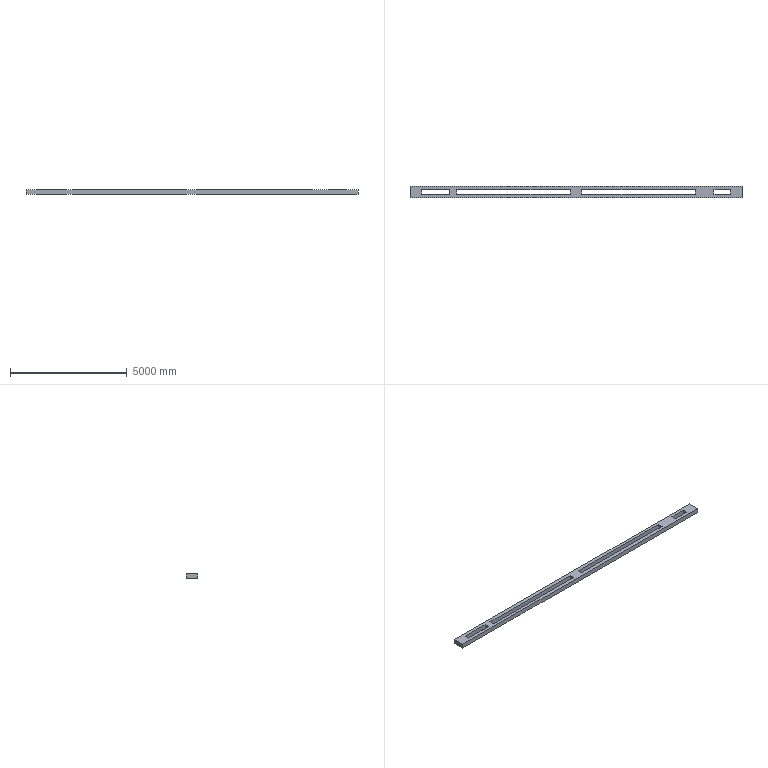Part | SolidWorks | features ICE 2, Extrusion 1 | 1 solid | 22 faces | box 14220 x 500 x 200 mm | volume 957200000 mm3 | plane 22
STEP:
#1=CARTESIAN_POINT('',(-7110.,250.,0.));
#2=VERTEX_POINT('',#1);
#3=CARTESIAN_POINT('',(-7110.,-250.,0.));
#4=VERTEX_POINT('',#3);
#5=CARTESIAN_POINT('',(-7110.,-250.,0.));
#6=DIRECTION('',(0.,-1.,0.));
#7=VECTOR('',#6,1000.);
#8=LINE('',#5,#7);
#9=EDGE_CURVE('',#2,#4,#8,.T.);
#10=ORIENTED_EDGE('',*,*,#9,.T.);
#11=CARTESIAN_POINT('',(-7110.,-250.,200.));
#12=VERTEX_POINT('',#11);
#13=CARTESIAN_POINT('',(-7110.,-250.,200.));
#14=DIRECTION('',(0.,0.,-1.));
#15=VECTOR('',#14,1000.);
#16=LINE('',#13,#15);
#17=EDGE_CURVE('',#12,#4,#16,.T.);
#18=ORIENTED_EDGE('',*,*,#17,.F.);
#19=CARTESIAN_POINT('',(-7110.,250.,200.));
#20=VERTEX_POINT('',#19);
#21=CARTESIAN_POINT('',(-7110.,-250.,200.));
#22=DIRECTION('',(0.,-1.,0.));
#23=VECTOR('',#22,1000.);
#24=LINE('',#21,#23);
#25=EDGE_CURVE('',#20,#12,#24,.T.);
#26=ORIENTED_EDGE('',*,*,#25,.F.);
#27=CARTESIAN_POINT('',(-7110.,250.,200.));
#28=DIRECTION('',(0.,0.,-1.));
#29=VECTOR('',#28,1000.);
#30=LINE('',#27,#29);
#31=EDGE_CURVE('',#20,#2,#30,.T.);
#32=ORIENTED_EDGE('',*,*,#31,.T.);
#33=EDGE_LOOP('',(#10,#18,#26,#32));
#34=FACE_OUTER_BOUND('',#33,.T.);
#35=CARTESIAN_POINT('',(-7110.,-250.,200.));
#36=DIRECTION('',(1.,0.,0.));
#37=DIRECTION('',(0.,0.,-1.));
#38=AXIS2_PLACEMENT_3D('',#35,#36,#37);
#39=PLANE('',#38);
#40=ADVANCED_FACE('',(#34),#39,.F.);
#41=CARTESIAN_POINT('',(7110.,-250.,0.));
#42=VERTEX_POINT('',#41);
#43=CARTESIAN_POINT('',(7110.,-250.,0.));
#44=DIRECTION('',(1.,0.,0.));
#45=VECTOR('',#44,1000.);
#46=LINE('',#43,#45);
#47=EDGE_CURVE('',#4,#42,#46,.T.);
#48=ORIENTED_EDGE('',*,*,#47,.T.);
#49=CARTESIAN_POINT('',(7110.,-250.,200.));
#50=VERTEX_POINT('',#49);
#51=CARTESIAN_POINT('',(7110.,-250.,200.));
#52=DIRECTION('',(0.,0.,-1.));
#53=VECTOR('',#52,1000.);
#54=LINE('',#51,#53);
#55=EDGE_CURVE('',#50,#42,#54,.T.);
#56=ORIENTED_EDGE('',*,*,#55,.F.);
#57=CARTESIAN_POINT('',(7110.,-250.,200.));
#58=DIRECTION('',(1.,0.,0.));
#59=VECTOR('',#58,1000.);
#60=LINE('',#57,#59);
#61=EDGE_CURVE('',#12,#50,#60,.T.);
#62=ORIENTED_EDGE('',*,*,#61,.F.);
#63=ORIENTED_EDGE('',*,*,#17,.T.);
#64=EDGE_LOOP('',(#48,#56,#62,#63));
#65=FACE_OUTER_BOUND('',#64,.T.);
#66=CARTESIAN_POINT('',(7110.,-250.,200.));
#67=DIRECTION('',(0.,1.,0.));
#68=DIRECTION('',(-1.,0.,0.));
#69=AXIS2_PLACEMENT_3D('',#66,#67,#68);
#70=PLANE('',#69);
#71=ADVANCED_FACE('',(#65),#70,.F.);
#72=CARTESIAN_POINT('',(7110.,250.,0.));
#73=VERTEX_POINT('',#72);
#74=CARTESIAN_POINT('',(7110.,-250.,0.));
#75=DIRECTION('',(0.,1.,0.));
#76=VECTOR('',#75,1000.);
#77=LINE('',#74,#76);
#78=EDGE_CURVE('',#42,#73,#77,.T.);
#79=ORIENTED_EDGE('',*,*,#78,.T.);
#80=CARTESIAN_POINT('',(7110.,250.,200.));
#81=VERTEX_POINT('',#80);
#82=CARTESIAN_POINT('',(7110.,250.,200.));
#83=DIRECTION('',(0.,0.,-1.));
#84=VECTOR('',#83,1000.);
#85=LINE('',#82,#84);
#86=EDGE_CURVE('',#81,#73,#85,.T.);
#87=ORIENTED_EDGE('',*,*,#86,.F.);
#88=CARTESIAN_POINT('',(7110.,-250.,200.));
#89=DIRECTION('',(0.,1.,0.));
#90=VECTOR('',#89,1000.);
#91=LINE('',#88,#90);
#92=EDGE_CURVE('',#50,#81,#91,.T.);
#93=ORIENTED_EDGE('',*,*,#92,.F.);
#94=ORIENTED_EDGE('',*,*,#55,.T.);
#95=EDGE_LOOP('',(#79,#87,#93,#94));
#96=FACE_OUTER_BOUND('',#95,.T.);
#97=CARTESIAN_POINT('',(7110.,-250.,200.));
#98=DIRECTION('',(-1.,0.,0.));
#99=DIRECTION('',(0.,0.,1.));
#100=AXIS2_PLACEMENT_3D('',#97,#98,#99);
#101=PLANE('',#100);
#102=ADVANCED_FACE('',(#96),#101,.F.);
#103=CARTESIAN_POINT('',(7110.,250.,0.));
#104=DIRECTION('',(-1.,0.,0.));
#105=VECTOR('',#104,1000.);
#106=LINE('',#103,#105);
#107=EDGE_CURVE('',#73,#2,#106,.T.);
#108=ORIENTED_EDGE('',*,*,#107,.T.);
#109=ORIENTED_EDGE('',*,*,#31,.F.);
#110=CARTESIAN_POINT('',(7110.,250.,200.));
#111=DIRECTION('',(-1.,0.,0.));
#112=VECTOR('',#111,1000.);
#113=LINE('',#110,#112);
#114=EDGE_CURVE('',#81,#20,#113,.T.);
#115=ORIENTED_EDGE('',*,*,#114,.F.);
#116=ORIENTED_EDGE('',*,*,#86,.T.);
#117=EDGE_LOOP('',(#108,#109,#115,#116));
#118=FACE_OUTER_BOUND('',#117,.T.);
#119=CARTESIAN_POINT('',(7110.,250.,200.));
#120=DIRECTION('',(0.,-1.,0.));
#121=DIRECTION('',(1.,0.,0.));
#122=AXIS2_PLACEMENT_3D('',#119,#120,#121);
#123=PLANE('',#122);
#124=ADVANCED_FACE('',(#118),#123,.F.);
#125=CARTESIAN_POINT('',(5910.,-100.,200.));
#126=VERTEX_POINT('',#125);
#127=CARTESIAN_POINT('',(6610.,-100.,200.));
#128=VERTEX_POINT('',#127);
#129=CARTESIAN_POINT('',(6610.,-100.,200.));
#130=DIRECTION('',(1.,0.,0.));
#131=VECTOR('',#130,1000.);
#132=LINE('',#129,#131);
#133=EDGE_CURVE('',#126,#128,#132,.T.);
#134=ORIENTED_EDGE('',*,*,#133,.F.);
#135=CARTESIAN_POINT('',(5910.,100.,200.));
#136=VERTEX_POINT('',#135);
#137=CARTESIAN_POINT('',(5910.,100.,200.));
#138=DIRECTION('',(0.,1.,0.));
#139=VECTOR('',#138,1000.);
#140=LINE('',#137,#139);
#141=EDGE_CURVE('',#126,#136,#140,.T.);
#142=ORIENTED_EDGE('',*,*,#141,.T.);
#143=CARTESIAN_POINT('',(6610.,100.,200.));
#144=VERTEX_POINT('',#143);
#145=CARTESIAN_POINT('',(6610.,100.,200.));
#146=DIRECTION('',(-1.,0.,0.));
#147=VECTOR('',#146,1000.);
#148=LINE('',#145,#147);
#149=EDGE_CURVE('',#144,#136,#148,.T.);
#150=ORIENTED_EDGE('',*,*,#149,.F.);
#151=CARTESIAN_POINT('',(6610.,100.,200.));
#152=DIRECTION('',(0.,1.,0.));
#153=VECTOR('',#152,1000.);
#154=LINE('',#151,#153);
#155=EDGE_CURVE('',#128,#144,#154,.T.);
#156=ORIENTED_EDGE('',*,*,#155,.F.);
#157=EDGE_LOOP('',(#134,#142,#150,#156));
#158=FACE_BOUND('',#157,.T.);
#159=CARTESIAN_POINT('',(-6610.,100.,200.));
#160=VERTEX_POINT('',#159);
#161=CARTESIAN_POINT('',(-6610.,-100.,200.));
#162=VERTEX_POINT('',#161);
#163=CARTESIAN_POINT('',(-6610.,100.,200.));
#164=DIRECTION('',(0.,-1.,0.));
#165=VECTOR('',#164,1000.);
#166=LINE('',#163,#165);
#167=EDGE_CURVE('',#160,#162,#166,.T.);
#168=ORIENTED_EDGE('',*,*,#167,.F.);
#169=CARTESIAN_POINT('',(-5410.,100.,200.));
#170=VERTEX_POINT('',#169);
#171=CARTESIAN_POINT('',(-6610.,100.,200.));
#172=DIRECTION('',(-1.,0.,0.));
#173=VECTOR('',#172,1000.);
#174=LINE('',#171,#173);
#175=EDGE_CURVE('',#170,#160,#174,.T.);
#176=ORIENTED_EDGE('',*,*,#175,.F.);
#177=CARTESIAN_POINT('',(-5410.,-100.,200.));
#178=VERTEX_POINT('',#177);
#179=CARTESIAN_POINT('',(-5410.,100.,200.));
#180=DIRECTION('',(0.,1.,0.));
#181=VECTOR('',#180,1000.);
#182=LINE('',#179,#181);
#183=EDGE_CURVE('',#178,#170,#182,.T.);
#184=ORIENTED_EDGE('',*,*,#183,.F.);
#185=CARTESIAN_POINT('',(-6610.,-100.,200.));
#186=DIRECTION('',(1.,0.,0.));
#187=VECTOR('',#186,1000.);
#188=LINE('',#185,#187);
#189=EDGE_CURVE('',#162,#178,#188,.T.);
#190=ORIENTED_EDGE('',*,*,#189,.F.);
#191=EDGE_LOOP('',(#168,#176,#184,#190));
#192=FACE_BOUND('',#191,.T.);
#193=CARTESIAN_POINT('',(-5110.,100.,200.));
#194=VERTEX_POINT('',#193);
#195=CARTESIAN_POINT('',(-5110.,-100.,200.));
#196=VERTEX_POINT('',#195);
#197=CARTESIAN_POINT('',(-5110.,100.,200.));
#198=DIRECTION('',(0.,-1.,0.));
#199=VECTOR('',#198,1000.);
#200=LINE('',#197,#199);
#201=EDGE_CURVE('',#194,#196,#200,.T.);
#202=ORIENTED_EDGE('',*,*,#201,.F.);
#203=CARTESIAN_POINT('',(-250.,100.,200.));
#204=VERTEX_POINT('',#203);
#205=CARTESIAN_POINT('',(-5110.,100.,200.));
#206=DIRECTION('',(-1.,0.,0.));
#207=VECTOR('',#206,1000.);
#208=LINE('',#205,#207);
#209=EDGE_CURVE('',#204,#194,#208,.T.);
#210=ORIENTED_EDGE('',*,*,#209,.F.);
#211=CARTESIAN_POINT('',(-250.,-100.,200.));
#212=VERTEX_POINT('',#211);
#213=CARTESIAN_POINT('',(-250.,100.,200.));
#214=DIRECTION('',(0.,1.,0.));
#215=VECTOR('',#214,1000.);
#216=LINE('',#213,#215);
#217=EDGE_CURVE('',#212,#204,#216,.T.);
#218=ORIENTED_EDGE('',*,*,#217,.F.);
#219=CARTESIAN_POINT('',(-5110.,-100.,200.));
#220=DIRECTION('',(1.,0.,0.));
#221=VECTOR('',#220,1000.);
#222=LINE('',#219,#221);
#223=EDGE_CURVE('',#196,#212,#222,.T.);
#224=ORIENTED_EDGE('',*,*,#223,.F.);
#225=EDGE_LOOP('',(#202,#210,#218,#224));
#226=FACE_BOUND('',#225,.T.);
#227=CARTESIAN_POINT('',(5110.,100.,200.));
#228=VERTEX_POINT('',#227);
#229=CARTESIAN_POINT('',(250.,100.,200.));
#230=VERTEX_POINT('',#229);
#231=CARTESIAN_POINT('',(5110.,100.,200.));
#232=DIRECTION('',(-1.,0.,0.));
#233=VECTOR('',#232,1000.);
#234=LINE('',#231,#233);
#235=EDGE_CURVE('',#228,#230,#234,.T.);
#236=ORIENTED_EDGE('',*,*,#235,.F.);
#237=CARTESIAN_POINT('',(5110.,-100.,200.));
#238=VERTEX_POINT('',#237);
#239=CARTESIAN_POINT('',(5110.,100.,200.));
#240=DIRECTION('',(0.,1.,0.));
#241=VECTOR('',#240,1000.);
#242=LINE('',#239,#241);
#243=EDGE_CURVE('',#238,#228,#242,.T.);
#244=ORIENTED_EDGE('',*,*,#243,.F.);
#245=CARTESIAN_POINT('',(250.,-100.,200.));
#246=VERTEX_POINT('',#245);
#247=CARTESIAN_POINT('',(5110.,-100.,200.));
#248=DIRECTION('',(1.,0.,0.));
#249=VECTOR('',#248,1000.);
#250=LINE('',#247,#249);
#251=EDGE_CURVE('',#246,#238,#250,.T.);
#252=ORIENTED_EDGE('',*,*,#251,.F.);
#253=CARTESIAN_POINT('',(250.,100.,200.));
#254=DIRECTION('',(0.,-1.,0.));
#255=VECTOR('',#254,1000.);
#256=LINE('',#253,#255);
#257=EDGE_CURVE('',#230,#246,#256,.T.);
#258=ORIENTED_EDGE('',*,*,#257,.F.);
#259=EDGE_LOOP('',(#236,#244,#252,#258));
#260=FACE_BOUND('',#259,.T.);
#261=ORIENTED_EDGE('',*,*,#25,.T.);
#262=ORIENTED_EDGE('',*,*,#61,.T.);
#263=ORIENTED_EDGE('',*,*,#92,.T.);
#264=ORIENTED_EDGE('',*,*,#114,.T.);
#265=EDGE_LOOP('',(#261,#262,#263,#264));
#266=FACE_OUTER_BOUND('',#265,.T.);
#267=CARTESIAN_POINT('',(0.,0.,200.));
#268=DIRECTION('',(0.,0.,1.));
#269=DIRECTION('',(1.,0.,0.));
#270=AXIS2_PLACEMENT_3D('',#267,#268,#269);
#271=PLANE('',#270);
#272=ADVANCED_FACE('',(#158,#192,#226,#260,#266),#271,.T.);
#273=CARTESIAN_POINT('',(6610.,100.,0.));
#274=VERTEX_POINT('',#273);
#275=CARTESIAN_POINT('',(5910.,100.,0.));
#276=VERTEX_POINT('',#275);
#277=CARTESIAN_POINT('',(6610.,100.,0.));
#278=DIRECTION('',(-1.,0.,0.));
#279=VECTOR('',#278,1000.);
#280=LINE('',#277,#279);
#281=EDGE_CURVE('',#274,#276,#280,.T.);
#282=ORIENTED_EDGE('',*,*,#281,.T.);
#283=CARTESIAN_POINT('',(5910.,-100.,0.));
#284=VERTEX_POINT('',#283);
#285=CARTESIAN_POINT('',(5910.,100.,0.));
#286=DIRECTION('',(0.,-1.,0.));
#287=VECTOR('',#286,1000.);
#288=LINE('',#285,#287);
#289=EDGE_CURVE('',#276,#284,#288,.T.);
#290=ORIENTED_EDGE('',*,*,#289,.T.);
#291=CARTESIAN_POINT('',(6610.,-100.,0.));
#292=VERTEX_POINT('',#291);
#293=CARTESIAN_POINT('',(6610.,-100.,0.));
#294=DIRECTION('',(1.,0.,0.));
#295=VECTOR('',#294,1000.);
#296=LINE('',#293,#295);
#297=EDGE_CURVE('',#284,#292,#296,.T.);
#298=ORIENTED_EDGE('',*,*,#297,.T.);
#299=CARTESIAN_POINT('',(6610.,100.,0.));
#300=DIRECTION('',(0.,1.,0.));
#301=VECTOR('',#300,1000.);
#302=LINE('',#299,#301);
#303=EDGE_CURVE('',#292,#274,#302,.T.);
#304=ORIENTED_EDGE('',*,*,#303,.T.);
#305=EDGE_LOOP('',(#282,#290,#298,#304));
#306=FACE_BOUND('',#305,.T.);
#307=CARTESIAN_POINT('',(-5410.,100.,0.));
#308=VERTEX_POINT('',#307);
#309=CARTESIAN_POINT('',(-6610.,100.,0.));
#310=VERTEX_POINT('',#309);
#311=CARTESIAN_POINT('',(-6610.,100.,0.));
#312=DIRECTION('',(-1.,0.,0.));
#313=VECTOR('',#312,1000.);
#314=LINE('',#311,#313);
#315=EDGE_CURVE('',#308,#310,#314,.T.);
#316=ORIENTED_EDGE('',*,*,#315,.T.);
#317=CARTESIAN_POINT('',(-6610.,-100.,0.));
#318=VERTEX_POINT('',#317);
#319=CARTESIAN_POINT('',(-6610.,100.,0.));
#320=DIRECTION('',(0.,-1.,0.));
#321=VECTOR('',#320,1000.);
#322=LINE('',#319,#321);
#323=EDGE_CURVE('',#310,#318,#322,.T.);
#324=ORIENTED_EDGE('',*,*,#323,.T.);
#325=CARTESIAN_POINT('',(-5410.,-100.,0.));
#326=VERTEX_POINT('',#325);
#327=CARTESIAN_POINT('',(-6610.,-100.,0.));
#328=DIRECTION('',(1.,0.,0.));
#329=VECTOR('',#328,1000.);
#330=LINE('',#327,#329);
#331=EDGE_CURVE('',#318,#326,#330,.T.);
#332=ORIENTED_EDGE('',*,*,#331,.T.);
#333=CARTESIAN_POINT('',(-5410.,100.,0.));
#334=DIRECTION('',(0.,1.,0.));
#335=VECTOR('',#334,1000.);
#336=LINE('',#333,#335);
#337=EDGE_CURVE('',#326,#308,#336,.T.);
#338=ORIENTED_EDGE('',*,*,#337,.T.);
#339=EDGE_LOOP('',(#316,#324,#332,#338));
#340=FACE_BOUND('',#339,.T.);
#341=CARTESIAN_POINT('',(-250.,100.,0.));
#342=VERTEX_POINT('',#341);
#343=CARTESIAN_POINT('',(-5110.,100.,0.));
#344=VERTEX_POINT('',#343);
#345=CARTESIAN_POINT('',(-5110.,100.,0.));
#346=DIRECTION('',(-1.,0.,0.));
#347=VECTOR('',#346,1000.);
#348=LINE('',#345,#347);
#349=EDGE_CURVE('',#342,#344,#348,.T.);
#350=ORIENTED_EDGE('',*,*,#349,.T.);
#351=CARTESIAN_POINT('',(-5110.,-100.,0.));
#352=VERTEX_POINT('',#351);
#353=CARTESIAN_POINT('',(-5110.,100.,0.));
#354=DIRECTION('',(0.,-1.,0.));
#355=VECTOR('',#354,1000.);
#356=LINE('',#353,#355);
#357=EDGE_CURVE('',#344,#352,#356,.T.);
#358=ORIENTED_EDGE('',*,*,#357,.T.);
#359=CARTESIAN_POINT('',(-250.,-100.,0.));
#360=VERTEX_POINT('',#359);
#361=CARTESIAN_POINT('',(-5110.,-100.,0.));
#362=DIRECTION('',(1.,0.,0.));
#363=VECTOR('',#362,1000.);
#364=LINE('',#361,#363);
#365=EDGE_CURVE('',#352,#360,#364,.T.);
#366=ORIENTED_EDGE('',*,*,#365,.T.);
#367=CARTESIAN_POINT('',(-250.,100.,0.));
#368=DIRECTION('',(0.,1.,0.));
#369=VECTOR('',#368,1000.);
#370=LINE('',#367,#369);
#371=EDGE_CURVE('',#360,#342,#370,.T.);
#372=ORIENTED_EDGE('',*,*,#371,.T.);
#373=EDGE_LOOP('',(#350,#358,#366,#372));
#374=FACE_BOUND('',#373,.T.);
#375=CARTESIAN_POINT('',(5110.,-100.,0.));
#376=VERTEX_POINT('',#375);
#377=CARTESIAN_POINT('',(5110.,100.,0.));
#378=VERTEX_POINT('',#377);
#379=CARTESIAN_POINT('',(5110.,100.,0.));
#380=DIRECTION('',(0.,1.,0.));
#381=VECTOR('',#380,1000.);
#382=LINE('',#379,#381);
#383=EDGE_CURVE('',#376,#378,#382,.T.);
#384=ORIENTED_EDGE('',*,*,#383,.T.);
#385=CARTESIAN_POINT('',(250.,100.,0.));
#386=VERTEX_POINT('',#385);
#387=CARTESIAN_POINT('',(5110.,100.,0.));
#388=DIRECTION('',(-1.,0.,0.));
#389=VECTOR('',#388,1000.);
#390=LINE('',#387,#389);
#391=EDGE_CURVE('',#378,#386,#390,.T.);
#392=ORIENTED_EDGE('',*,*,#391,.T.);
#393=CARTESIAN_POINT('',(250.,-100.,0.));
#394=VERTEX_POINT('',#393);
#395=CARTESIAN_POINT('',(250.,100.,0.));
#396=DIRECTION('',(0.,-1.,0.));
#397=VECTOR('',#396,1000.);
#398=LINE('',#395,#397);
#399=EDGE_CURVE('',#386,#394,#398,.T.);
#400=ORIENTED_EDGE('',*,*,#399,.T.);
#401=CARTESIAN_POINT('',(5110.,-100.,0.));
#402=DIRECTION('',(1.,0.,0.));
#403=VECTOR('',#402,1000.);
#404=LINE('',#401,#403);
#405=EDGE_CURVE('',#394,#376,#404,.T.);
#406=ORIENTED_EDGE('',*,*,#405,.T.);
#407=EDGE_LOOP('',(#384,#392,#400,#406));
#408=FACE_BOUND('',#407,.T.);
#409=ORIENTED_EDGE('',*,*,#9,.F.);
#410=ORIENTED_EDGE('',*,*,#107,.F.);
#411=ORIENTED_EDGE('',*,*,#78,.F.);
#412=ORIENTED_EDGE('',*,*,#47,.F.);
#413=EDGE_LOOP('',(#409,#410,#411,#412));
#414=FACE_OUTER_BOUND('',#413,.T.);
#415=CARTESIAN_POINT('',(0.,0.,0.));
#416=DIRECTION('',(0.,0.,1.));
#417=DIRECTION('',(1.,0.,0.));
#418=AXIS2_PLACEMENT_3D('',#415,#416,#417);
#419=PLANE('',#418);
#420=ADVANCED_FACE('',(#306,#340,#374,#408,#414),#419,.F.);
#421=ORIENTED_EDGE('',*,*,#149,.T.);
#422=CARTESIAN_POINT('',(5910.,100.,-538.516));
#423=DIRECTION('',(0.,0.,1.));
#424=VECTOR('',#423,1000.);
#425=LINE('',#422,#424);
#426=EDGE_CURVE('',#276,#136,#425,.T.);
#427=ORIENTED_EDGE('',*,*,#426,.F.);
#428=ORIENTED_EDGE('',*,*,#281,.F.);
#429=CARTESIAN_POINT('',(6610.,100.,0.));
#430=DIRECTION('',(0.,0.,1.));
#431=VECTOR('',#430,1000.);
#432=LINE('',#429,#431);
#433=EDGE_CURVE('',#274,#144,#432,.T.);
#434=ORIENTED_EDGE('',*,*,#433,.T.);
#435=EDGE_LOOP('',(#421,#427,#428,#434));
#436=FACE_OUTER_BOUND('',#435,.T.);
#437=CARTESIAN_POINT('',(6610.,100.,0.));
#438=DIRECTION('',(0.,1.,0.));
#439=DIRECTION('',(0.,0.,1.));
#440=AXIS2_PLACEMENT_3D('',#437,#438,#439);
#441=PLANE('',#440);
#442=ADVANCED_FACE('',(#436),#441,.F.);
#443=ORIENTED_EDGE('',*,*,#155,.T.);
#444=ORIENTED_EDGE('',*,*,#433,.F.);
#445=ORIENTED_EDGE('',*,*,#303,.F.);
#446=CARTESIAN_POINT('',(6610.,-100.,0.));
#447=DIRECTION('',(0.,0.,1.));
#448=VECTOR('',#447,1000.);
#449=LINE('',#446,#448);
#450=EDGE_CURVE('',#292,#128,#449,.T.);
#451=ORIENTED_EDGE('',*,*,#450,.T.);
#452=EDGE_LOOP('',(#443,#444,#445,#451));
#453=FACE_OUTER_BOUND('',#452,.T.);
#454=CARTESIAN_POINT('',(6610.,100.,0.));
#455=DIRECTION('',(1.,0.,0.));
#456=DIRECTION('',(0.,0.,-1.));
#457=AXIS2_PLACEMENT_3D('',#454,#455,#456);
#458=PLANE('',#457);
#459=ADVANCED_FACE('',(#453),#458,.F.);
#460=ORIENTED_EDGE('',*,*,#297,.F.);
#461=CARTESIAN_POINT('',(5910.,-100.,-538.516));
#462=DIRECTION('',(0.,0.,1.));
#463=VECTOR('',#462,1000.);
#464=LINE('',#461,#463);
#465=EDGE_CURVE('',#284,#126,#464,.T.);
#466=ORIENTED_EDGE('',*,*,#465,.T.);
#467=ORIENTED_EDGE('',*,*,#133,.T.);
#468=ORIENTED_EDGE('',*,*,#450,.F.);
#469=EDGE_LOOP('',(#460,#466,#467,#468));
#470=FACE_OUTER_BOUND('',#469,.T.);
#471=CARTESIAN_POINT('',(6610.,-100.,0.));
#472=DIRECTION('',(0.,-1.,0.));
#473=DIRECTION('',(0.,0.,-1.));
#474=AXIS2_PLACEMENT_3D('',#471,#472,#473);
#475=PLANE('',#474);
#476=ADVANCED_FACE('',(#470),#475,.F.);
#477=ORIENTED_EDGE('',*,*,#235,.T.);
#478=CARTESIAN_POINT('',(250.,100.,0.));
#479=DIRECTION('',(0.,0.,1.));
#480=VECTOR('',#479,1000.);
#481=LINE('',#478,#480);
#482=EDGE_CURVE('',#386,#230,#481,.T.);
#483=ORIENTED_EDGE('',*,*,#482,.F.);
#484=ORIENTED_EDGE('',*,*,#391,.F.);
#485=CARTESIAN_POINT('',(5110.,100.,0.));
#486=DIRECTION('',(0.,0.,1.));
#487=VECTOR('',#486,1000.);
#488=LINE('',#485,#487);
#489=EDGE_CURVE('',#378,#228,#488,.T.);
#490=ORIENTED_EDGE('',*,*,#489,.T.);
#491=EDGE_LOOP('',(#477,#483,#484,#490));
#492=FACE_OUTER_BOUND('',#491,.T.);
#493=CARTESIAN_POINT('',(5110.,100.,0.));
#494=DIRECTION('',(0.,1.,0.));
#495=DIRECTION('',(0.,0.,1.));
#496=AXIS2_PLACEMENT_3D('',#493,#494,#495);
#497=PLANE('',#496);
#498=ADVANCED_FACE('',(#492),#497,.F.);
#499=ORIENTED_EDGE('',*,*,#243,.T.);
#500=ORIENTED_EDGE('',*,*,#489,.F.);
#501=ORIENTED_EDGE('',*,*,#383,.F.);
#502=CARTESIAN_POINT('',(5110.,-100.,0.));
#503=DIRECTION('',(0.,0.,1.));
#504=VECTOR('',#503,1000.);
#505=LINE('',#502,#504);
#506=EDGE_CURVE('',#376,#238,#505,.T.);
#507=ORIENTED_EDGE('',*,*,#506,.T.);
#508=EDGE_LOOP('',(#499,#500,#501,#507));
#509=FACE_OUTER_BOUND('',#508,.T.);
#510=CARTESIAN_POINT('',(5110.,100.,0.));
#511=DIRECTION('',(1.,0.,0.));
#512=DIRECTION('',(0.,0.,-1.));
#513=AXIS2_PLACEMENT_3D('',#510,#511,#512);
#514=PLANE('',#513);
#515=ADVANCED_FACE('',(#509),#514,.F.);
#516=ORIENTED_EDGE('',*,*,#251,.T.);
#517=ORIENTED_EDGE('',*,*,#506,.F.);
#518=ORIENTED_EDGE('',*,*,#405,.F.);
#519=CARTESIAN_POINT('',(250.,-100.,0.));
#520=DIRECTION('',(0.,0.,1.));
#521=VECTOR('',#520,1000.);
#522=LINE('',#519,#521);
#523=EDGE_CURVE('',#394,#246,#522,.T.);
#524=ORIENTED_EDGE('',*,*,#523,.T.);
#525=EDGE_LOOP('',(#516,#517,#518,#524));
#526=FACE_OUTER_BOUND('',#525,.T.);
#527=CARTESIAN_POINT('',(5110.,-100.,0.));
#528=DIRECTION('',(0.,-1.,0.));
#529=DIRECTION('',(0.,0.,-1.));
#530=AXIS2_PLACEMENT_3D('',#527,#528,#529);
#531=PLANE('',#530);
#532=ADVANCED_FACE('',(#526),#531,.F.);
#533=ORIENTED_EDGE('',*,*,#257,.T.);
#534=ORIENTED_EDGE('',*,*,#523,.F.);
#535=ORIENTED_EDGE('',*,*,#399,.F.);
#536=ORIENTED_EDGE('',*,*,#482,.T.);
#537=EDGE_LOOP('',(#533,#534,#535,#536));
#538=FACE_OUTER_BOUND('',#537,.T.);
#539=CARTESIAN_POINT('',(250.,100.,0.));
#540=DIRECTION('',(-1.,0.,0.));
#541=DIRECTION('',(0.,0.,1.));
#542=AXIS2_PLACEMENT_3D('',#539,#540,#541);
#543=PLANE('',#542);
#544=ADVANCED_FACE('',(#538),#543,.F.);
#545=ORIENTED_EDGE('',*,*,#201,.T.);
#546=CARTESIAN_POINT('',(-5110.,-100.,0.));
#547=DIRECTION('',(0.,0.,1.));
#548=VECTOR('',#547,1000.);
#549=LINE('',#546,#548);
#550=EDGE_CURVE('',#352,#196,#549,.T.);
#551=ORIENTED_EDGE('',*,*,#550,.F.);
#552=ORIENTED_EDGE('',*,*,#357,.F.);
#553=CARTESIAN_POINT('',(-5110.,100.,0.));
#554=DIRECTION('',(0.,0.,1.));
#555=VECTOR('',#554,1000.);
#556=LINE('',#553,#555);
#557=EDGE_CURVE('',#344,#194,#556,.T.);
#558=ORIENTED_EDGE('',*,*,#557,.T.);
#559=EDGE_LOOP('',(#545,#551,#552,#558));
#560=FACE_OUTER_BOUND('',#559,.T.);
#561=CARTESIAN_POINT('',(-5110.,100.,0.));
#562=DIRECTION('',(-1.,0.,0.));
#563=DIRECTION('',(0.,0.,1.));
#564=AXIS2_PLACEMENT_3D('',#561,#562,#563);
#565=PLANE('',#564);
#566=ADVANCED_FACE('',(#560),#565,.F.);
#567=ORIENTED_EDGE('',*,*,#209,.T.);
#568=ORIENTED_EDGE('',*,*,#557,.F.);
#569=ORIENTED_EDGE('',*,*,#349,.F.);
#570=CARTESIAN_POINT('',(-250.,100.,0.));
#571=DIRECTION('',(0.,0.,1.));
#572=VECTOR('',#571,1000.);
#573=LINE('',#570,#572);
#574=EDGE_CURVE('',#342,#204,#573,.T.);
#575=ORIENTED_EDGE('',*,*,#574,.T.);
#576=EDGE_LOOP('',(#567,#568,#569,#575));
#577=FACE_OUTER_BOUND('',#576,.T.);
#578=CARTESIAN_POINT('',(-5110.,100.,0.));
#579=DIRECTION('',(0.,1.,0.));
#580=DIRECTION('',(0.,0.,1.));
#581=AXIS2_PLACEMENT_3D('',#578,#579,#580);
#582=PLANE('',#581);
#583=ADVANCED_FACE('',(#577),#582,.F.);
#584=ORIENTED_EDGE('',*,*,#217,.T.);
#585=ORIENTED_EDGE('',*,*,#574,.F.);
#586=ORIENTED_EDGE('',*,*,#371,.F.);
#587=CARTESIAN_POINT('',(-250.,-100.,0.));
#588=DIRECTION('',(0.,0.,1.));
#589=VECTOR('',#588,1000.);
#590=LINE('',#587,#589);
#591=EDGE_CURVE('',#360,#212,#590,.T.);
#592=ORIENTED_EDGE('',*,*,#591,.T.);
#593=EDGE_LOOP('',(#584,#585,#586,#592));
#594=FACE_OUTER_BOUND('',#593,.T.);
#595=CARTESIAN_POINT('',(-250.,100.,0.));
#596=DIRECTION('',(1.,0.,0.));
#597=DIRECTION('',(0.,0.,-1.));
#598=AXIS2_PLACEMENT_3D('',#595,#596,#597);
#599=PLANE('',#598);
#600=ADVANCED_FACE('',(#594),#599,.F.);
#601=ORIENTED_EDGE('',*,*,#223,.T.);
#602=ORIENTED_EDGE('',*,*,#591,.F.);
#603=ORIENTED_EDGE('',*,*,#365,.F.);
#604=ORIENTED_EDGE('',*,*,#550,.T.);
#605=EDGE_LOOP('',(#601,#602,#603,#604));
#606=FACE_OUTER_BOUND('',#605,.T.);
#607=CARTESIAN_POINT('',(-5110.,-100.,0.));
#608=DIRECTION('',(0.,-1.,0.));
#609=DIRECTION('',(0.,0.,-1.));
#610=AXIS2_PLACEMENT_3D('',#607,#608,#609);
#611=PLANE('',#610);
#612=ADVANCED_FACE('',(#606),#611,.F.);
#613=ORIENTED_EDGE('',*,*,#167,.T.);
#614=CARTESIAN_POINT('',(-6610.,-100.,0.));
#615=DIRECTION('',(0.,0.,1.));
#616=VECTOR('',#615,1000.);
#617=LINE('',#614,#616);
#618=EDGE_CURVE('',#318,#162,#617,.T.);
#619=ORIENTED_EDGE('',*,*,#618,.F.);
#620=ORIENTED_EDGE('',*,*,#323,.F.);
#621=CARTESIAN_POINT('',(-6610.,100.,0.));
#622=DIRECTION('',(0.,0.,1.));
#623=VECTOR('',#622,1000.);
#624=LINE('',#621,#623);
#625=EDGE_CURVE('',#310,#160,#624,.T.);
#626=ORIENTED_EDGE('',*,*,#625,.T.);
#627=EDGE_LOOP('',(#613,#619,#620,#626));
#628=FACE_OUTER_BOUND('',#627,.T.);
#629=CARTESIAN_POINT('',(-6610.,100.,0.));
#630=DIRECTION('',(-1.,0.,0.));
#631=DIRECTION('',(0.,0.,1.));
#632=AXIS2_PLACEMENT_3D('',#629,#630,#631);
#633=PLANE('',#632);
#634=ADVANCED_FACE('',(#628),#633,.F.);
#635=ORIENTED_EDGE('',*,*,#175,.T.);
#636=ORIENTED_EDGE('',*,*,#625,.F.);
#637=ORIENTED_EDGE('',*,*,#315,.F.);
#638=CARTESIAN_POINT('',(-5410.,100.,0.));
#639=DIRECTION('',(0.,0.,1.));
#640=VECTOR('',#639,1000.);
#641=LINE('',#638,#640);
#642=EDGE_CURVE('',#308,#170,#641,.T.);
#643=ORIENTED_EDGE('',*,*,#642,.T.);
#644=EDGE_LOOP('',(#635,#636,#637,#643));
#645=FACE_OUTER_BOUND('',#644,.T.);
#646=CARTESIAN_POINT('',(-6610.,100.,0.));
#647=DIRECTION('',(0.,1.,0.));
#648=DIRECTION('',(0.,0.,1.));
#649=AXIS2_PLACEMENT_3D('',#646,#647,#648);
#650=PLANE('',#649);
#651=ADVANCED_FACE('',(#645),#650,.F.);
#652=ORIENTED_EDGE('',*,*,#183,.T.);
#653=ORIENTED_EDGE('',*,*,#642,.F.);
#654=ORIENTED_EDGE('',*,*,#337,.F.);
#655=CARTESIAN_POINT('',(-5410.,-100.,0.));
#656=DIRECTION('',(0.,0.,1.));
#657=VECTOR('',#656,1000.);
#658=LINE('',#655,#657);
#659=EDGE_CURVE('',#326,#178,#658,.T.);
#660=ORIENTED_EDGE('',*,*,#659,.T.);
#661=EDGE_LOOP('',(#652,#653,#654,#660));
#662=FACE_OUTER_BOUND('',#661,.T.);
#663=CARTESIAN_POINT('',(-5410.,100.,0.));
#664=DIRECTION('',(1.,0.,0.));
#665=DIRECTION('',(0.,0.,-1.));
#666=AXIS2_PLACEMENT_3D('',#663,#664,#665);
#667=PLANE('',#666);
#668=ADVANCED_FACE('',(#662),#667,.F.);
#669=ORIENTED_EDGE('',*,*,#189,.T.);
#670=ORIENTED_EDGE('',*,*,#659,.F.);
#671=ORIENTED_EDGE('',*,*,#331,.F.);
#672=ORIENTED_EDGE('',*,*,#618,.T.);
#673=EDGE_LOOP('',(#669,#670,#671,#672));
#674=FACE_OUTER_BOUND('',#673,.T.);
#675=CARTESIAN_POINT('',(-6610.,-100.,0.));
#676=DIRECTION('',(0.,-1.,0.));
#677=DIRECTION('',(0.,0.,-1.));
#678=AXIS2_PLACEMENT_3D('',#675,#676,#677);
#679=PLANE('',#678);
#680=ADVANCED_FACE('',(#674),#679,.F.);
#681=ORIENTED_EDGE('',*,*,#289,.F.);
#682=ORIENTED_EDGE('',*,*,#426,.T.);
#683=ORIENTED_EDGE('',*,*,#141,.F.);
#684=ORIENTED_EDGE('',*,*,#465,.F.);
#685=EDGE_LOOP('',(#681,#682,#683,#684));
#686=FACE_OUTER_BOUND('',#685,.T.);
#687=CARTESIAN_POINT('',(5910.,100.,-538.516));
#688=DIRECTION('',(1.,0.,0.));
#689=DIRECTION('',(0.,0.,-1.));
#690=AXIS2_PLACEMENT_3D('',#687,#688,#689);
#691=PLANE('',#690);
#692=ADVANCED_FACE('',(#686),#691,.T.);
#693=CLOSED_SHELL('',(#40,#71,#102,#124,#272,#420,#442,#459,#476,#498,#515,#532,#544,#566,#583,#600,#612,#634,#651,#668,#680,#692));
#694=MANIFOLD_SOLID_BREP('',#693);
#695=CARTESIAN_POINT('',(0.,0.,0.));
#696=DIRECTION('',(0.,0.,1.));
#697=DIRECTION('',(1.,0.,0.));
#698=AXIS2_PLACEMENT_3D('',#695,#696,#697);
#699=(LENGTH_UNIT()NAMED_UNIT(*)SI_UNIT(.MILLI.,.METRE.));
#700=UNCERTAINTY_MEASURE_WITH_UNIT(LENGTH_MEASURE(0.00001),#699,'','');
#701=(NAMED_UNIT(*)PLANE_ANGLE_UNIT()SI_UNIT($,.RADIAN.));
#702=(NAMED_UNIT(*)SI_UNIT($,.STERADIAN.)SOLID_ANGLE_UNIT());
#703=(GEOMETRIC_REPRESENTATION_CONTEXT(3)GLOBAL_UNCERTAINTY_ASSIGNED_CONTEXT((#700))GLOBAL_UNIT_ASSIGNED_CONTEXT((#699,#701,#702))REPRESENTATION_CONTEXT('',''));
#704=ADVANCED_BREP_SHAPE_REPRESENTATION('',(#694,#698),#703);